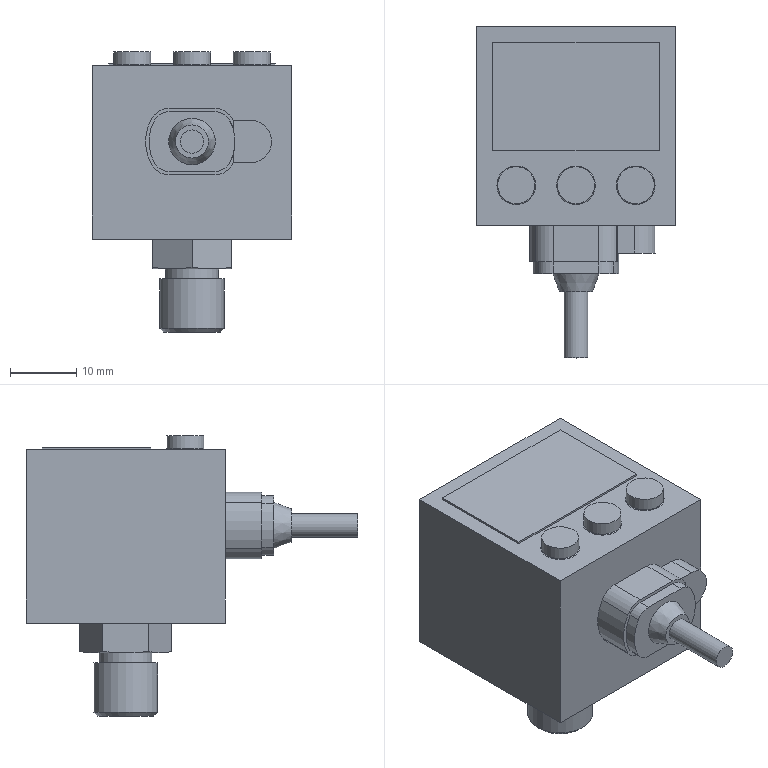Part | STEP file | _ZSE40AF-01-A_BODY(0).stp | 1 solid | 82 faces | box 30 x 50 x 42.2 mm | volume 26079 mm3 | plane 36 | cylinder 25 | cone 21 | commonest cylinder face diameters 5 x4 6 x4 5.6 x3 14 x3 2.459 x2 2.6 x2